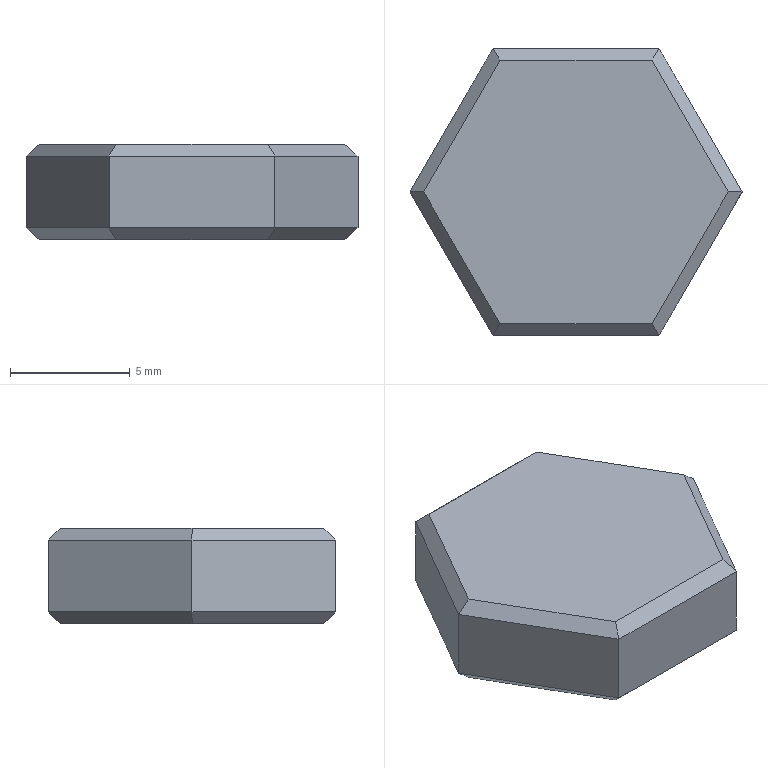Part | STEP file | Tube feed_id806_x_t | 1 solid | 20 faces | box 13.856 x 12 x 4 mm | volume 488.727 mm3 | plane 20
STEP:
#1=CARTESIAN_POINT('',(0.,0.,0.));
#2=DIRECTION('',(0.,0.,1.));
#3=DIRECTION('',(1.,0.,0.));
#4=AXIS2_PLACEMENT_3D('',#1,#2,#3);
#5=CARTESIAN_POINT('',(442.822,17.036,12.5));
#6=VERTEX_POINT('',#5);
#7=CARTESIAN_POINT('',(442.822,17.036,9.5));
#8=VERTEX_POINT('',#7);
#9=CARTESIAN_POINT('',(442.822,17.036,13.));
#10=DIRECTION('',(0.,0.,-1.));
#11=VECTOR('',#10,1.);
#12=LINE('',#9,#11);
#13=CARTESIAN_POINT('',(442.822,17.036,13.));
#14=DIRECTION('',(0.866,0.5,0.));
#15=DIRECTION('',(-0.5,0.866,0.));
#16=AXIS2_PLACEMENT_3D('',#13,#14,#15);
#17=PLANE('',#16);
#18=CARTESIAN_POINT('',(0.,0.));
#19=DIRECTION('',(0.,-1.));
#20=VECTOR('',#19,1.);
#21=LINE('',#18,#20);
#22=(GEOMETRIC_REPRESENTATION_CONTEXT(2)PARAMETRIC_REPRESENTATION_CONTEXT()REPRESENTATION_CONTEXT('',''));
#23=DEFINITIONAL_REPRESENTATION('',(#21),#22);
#24=PCURVE('',#17,#23);
#25=CARTESIAN_POINT('',(446.286,23.036,13.));
#26=DIRECTION('',(0.866,-0.5,0.));
#27=DIRECTION('',(0.5,0.866,0.));
#28=AXIS2_PLACEMENT_3D('',#25,#26,#27);
#29=PLANE('',#28);
#30=CARTESIAN_POINT('',(-6.928,0.));
#31=DIRECTION('',(0.,-1.));
#32=VECTOR('',#31,1.);
#33=LINE('',#30,#32);
#34=(GEOMETRIC_REPRESENTATION_CONTEXT(2)PARAMETRIC_REPRESENTATION_CONTEXT()REPRESENTATION_CONTEXT('',''));
#35=DEFINITIONAL_REPRESENTATION('',(#33),#34);
#36=PCURVE('',#29,#35);
#37=SURFACE_CURVE('',#12,(#24,#36),.PCURVE_S1.);
#38=EDGE_CURVE('',#6,#8,#37,.T.);
#39=ORIENTED_EDGE('',*,*,#38,.T.);
#40=CARTESIAN_POINT('',(446.286,11.036,9.5));
#41=VERTEX_POINT('',#40);
#42=CARTESIAN_POINT('',(442.822,17.036,9.5));
#43=DIRECTION('',(0.5,-0.866,0.));
#44=VECTOR('',#43,1.);
#45=LINE('',#42,#44);
#46=CARTESIAN_POINT('',(0.,-3.5));
#47=DIRECTION('',(-1.,0.));
#48=VECTOR('',#47,1.);
#49=LINE('',#46,#48);
#50=(GEOMETRIC_REPRESENTATION_CONTEXT(2)PARAMETRIC_REPRESENTATION_CONTEXT()REPRESENTATION_CONTEXT('',''));
#51=DEFINITIONAL_REPRESENTATION('',(#49),#50);
#52=PCURVE('',#17,#51);
#53=CARTESIAN_POINT('',(442.822,17.036,9.5));
#54=DIRECTION('',(0.6124,0.3536,0.7071));
#55=DIRECTION('',(0.5,-0.866,0.));
#56=AXIS2_PLACEMENT_3D('',#53,#54,#55);
#57=PLANE('',#56);
#58=CARTESIAN_POINT('',(0.,0.));
#59=DIRECTION('',(1.,0.));
#60=VECTOR('',#59,1.);
#61=LINE('',#58,#60);
#62=(GEOMETRIC_REPRESENTATION_CONTEXT(2)PARAMETRIC_REPRESENTATION_CONTEXT()REPRESENTATION_CONTEXT('',''));
#63=DEFINITIONAL_REPRESENTATION('',(#61),#62);
#64=PCURVE('',#57,#63);
#65=SURFACE_CURVE('',#45,(#52,#64),.PCURVE_S1.);
#66=EDGE_CURVE('',#8,#41,#65,.T.);
#67=ORIENTED_EDGE('',*,*,#66,.T.);
#68=CARTESIAN_POINT('',(446.286,11.036,12.5));
#69=VERTEX_POINT('',#68);
#70=CARTESIAN_POINT('',(446.286,11.036,13.));
#71=DIRECTION('',(0.,0.,-1.));
#72=VECTOR('',#71,1.);
#73=LINE('',#70,#72);
#74=CARTESIAN_POINT('',(-6.928,0.));
#75=DIRECTION('',(0.,-1.));
#76=VECTOR('',#75,1.);
#77=LINE('',#74,#76);
#78=(GEOMETRIC_REPRESENTATION_CONTEXT(2)PARAMETRIC_REPRESENTATION_CONTEXT()REPRESENTATION_CONTEXT('',''));
#79=DEFINITIONAL_REPRESENTATION('',(#77),#78);
#80=PCURVE('',#17,#79);
#81=CARTESIAN_POINT('',(446.286,11.036,13.));
#82=DIRECTION('',(0.,1.,0.));
#83=DIRECTION('',(-1.,0.,0.));
#84=AXIS2_PLACEMENT_3D('',#81,#82,#83);
#85=PLANE('',#84);
#86=CARTESIAN_POINT('',(0.,0.));
#87=DIRECTION('',(0.,-1.));
#88=VECTOR('',#87,1.);
#89=LINE('',#86,#88);
#90=(GEOMETRIC_REPRESENTATION_CONTEXT(2)PARAMETRIC_REPRESENTATION_CONTEXT()REPRESENTATION_CONTEXT('',''));
#91=DEFINITIONAL_REPRESENTATION('',(#89),#90);
#92=PCURVE('',#85,#91);
#93=SURFACE_CURVE('',#73,(#80,#92),.PCURVE_S1.);
#94=EDGE_CURVE('',#69,#41,#93,.T.);
#95=ORIENTED_EDGE('',*,*,#94,.F.);
#96=CARTESIAN_POINT('',(442.822,17.036,12.5));
#97=DIRECTION('',(-0.5,0.866,0.));
#98=VECTOR('',#97,1.);
#99=LINE('',#96,#98);
#100=CARTESIAN_POINT('',(0.,-0.5));
#101=DIRECTION('',(1.,0.));
#102=VECTOR('',#101,1.);
#103=LINE('',#100,#102);
#104=(GEOMETRIC_REPRESENTATION_CONTEXT(2)PARAMETRIC_REPRESENTATION_CONTEXT()REPRESENTATION_CONTEXT('',''));
#105=DEFINITIONAL_REPRESENTATION('',(#103),#104);
#106=PCURVE('',#17,#105);
#107=CARTESIAN_POINT('',(339.06,197.756,13.));
#108=DIRECTION('',(-0.6124,-0.3536,0.7071));
#109=DIRECTION('',(-0.5,0.866,0.));
#110=AXIS2_PLACEMENT_3D('',#107,#108,#109);
#111=PLANE('',#110);
#112=CARTESIAN_POINT('',(-208.39,0.7071));
#113=DIRECTION('',(1.,0.));
#114=VECTOR('',#113,1.);
#115=LINE('',#112,#114);
#116=(GEOMETRIC_REPRESENTATION_CONTEXT(2)PARAMETRIC_REPRESENTATION_CONTEXT()REPRESENTATION_CONTEXT('',''));
#117=DEFINITIONAL_REPRESENTATION('',(#115),#116);
#118=PCURVE('',#111,#117);
#119=SURFACE_CURVE('',#99,(#106,#118),.PCURVE_S1.);
#120=EDGE_CURVE('',#69,#6,#119,.T.);
#121=ORIENTED_EDGE('',*,*,#120,.T.);
#122=EDGE_LOOP('',(#39,#67,#95,#121));
#123=FACE_BOUND('',#122,.T.);
#124=ADVANCED_FACE('',(#123),#17,.F.);
#125=ORIENTED_EDGE('',*,*,#94,.T.);
#126=CARTESIAN_POINT('',(453.214,11.036,9.5));
#127=VERTEX_POINT('',#126);
#128=CARTESIAN_POINT('',(446.286,11.036,9.5));
#129=DIRECTION('',(1.,0.,0.));
#130=VECTOR('',#129,1.);
#131=LINE('',#128,#130);
#132=CARTESIAN_POINT('',(0.,-3.5));
#133=DIRECTION('',(-1.,0.));
#134=VECTOR('',#133,1.);
#135=LINE('',#132,#134);
#136=(GEOMETRIC_REPRESENTATION_CONTEXT(2)PARAMETRIC_REPRESENTATION_CONTEXT()REPRESENTATION_CONTEXT('',''));
#137=DEFINITIONAL_REPRESENTATION('',(#135),#136);
#138=PCURVE('',#85,#137);
#139=CARTESIAN_POINT('',(446.286,11.036,9.5));
#140=DIRECTION('',(0.,0.7071,0.7071));
#141=DIRECTION('',(1.,0.,0.));
#142=AXIS2_PLACEMENT_3D('',#139,#140,#141);
#143=PLANE('',#142);
#144=CARTESIAN_POINT('',(0.,0.));
#145=DIRECTION('',(1.,0.));
#146=VECTOR('',#145,1.);
#147=LINE('',#144,#146);
#148=(GEOMETRIC_REPRESENTATION_CONTEXT(2)PARAMETRIC_REPRESENTATION_CONTEXT()REPRESENTATION_CONTEXT('',''));
#149=DEFINITIONAL_REPRESENTATION('',(#147),#148);
#150=PCURVE('',#143,#149);
#151=SURFACE_CURVE('',#131,(#138,#150),.PCURVE_S1.);
#152=EDGE_CURVE('',#41,#127,#151,.T.);
#153=ORIENTED_EDGE('',*,*,#152,.T.);
#154=CARTESIAN_POINT('',(453.214,11.036,12.5));
#155=VERTEX_POINT('',#154);
#156=CARTESIAN_POINT('',(453.214,11.036,13.));
#157=DIRECTION('',(0.,0.,-1.));
#158=VECTOR('',#157,1.);
#159=LINE('',#156,#158);
#160=CARTESIAN_POINT('',(-6.928,0.));
#161=DIRECTION('',(0.,-1.));
#162=VECTOR('',#161,1.);
#163=LINE('',#160,#162);
#164=(GEOMETRIC_REPRESENTATION_CONTEXT(2)PARAMETRIC_REPRESENTATION_CONTEXT()REPRESENTATION_CONTEXT('',''));
#165=DEFINITIONAL_REPRESENTATION('',(#163),#164);
#166=PCURVE('',#85,#165);
#167=CARTESIAN_POINT('',(453.214,11.036,13.));
#168=DIRECTION('',(-0.866,0.5,0.));
#169=DIRECTION('',(-0.5,-0.866,0.));
#170=AXIS2_PLACEMENT_3D('',#167,#168,#169);
#171=PLANE('',#170);
#172=CARTESIAN_POINT('',(0.,0.));
#173=DIRECTION('',(0.,-1.));
#174=VECTOR('',#173,1.);
#175=LINE('',#172,#174);
#176=(GEOMETRIC_REPRESENTATION_CONTEXT(2)PARAMETRIC_REPRESENTATION_CONTEXT()REPRESENTATION_CONTEXT('',''));
#177=DEFINITIONAL_REPRESENTATION('',(#175),#176);
#178=PCURVE('',#171,#177);
#179=SURFACE_CURVE('',#159,(#166,#178),.PCURVE_S1.);
#180=EDGE_CURVE('',#155,#127,#179,.T.);
#181=ORIENTED_EDGE('',*,*,#180,.F.);
#182=CARTESIAN_POINT('',(446.286,11.036,12.5));
#183=DIRECTION('',(-1.,0.,0.));
#184=VECTOR('',#183,1.);
#185=LINE('',#182,#184);
#186=CARTESIAN_POINT('',(0.,-0.5));
#187=DIRECTION('',(1.,0.));
#188=VECTOR('',#187,1.);
#189=LINE('',#186,#188);
#190=(GEOMETRIC_REPRESENTATION_CONTEXT(2)PARAMETRIC_REPRESENTATION_CONTEXT()REPRESENTATION_CONTEXT('',''));
#191=DEFINITIONAL_REPRESENTATION('',(#189),#190);
#192=PCURVE('',#85,#191);
#193=CARTESIAN_POINT('',(0.,11.536,13.));
#194=DIRECTION('',(0.,-0.7071,0.7071));
#195=DIRECTION('',(-1.,0.,0.));
#196=AXIS2_PLACEMENT_3D('',#193,#194,#195);
#197=PLANE('',#196);
#198=CARTESIAN_POINT('',(-446.286,0.7071));
#199=DIRECTION('',(1.,0.));
#200=VECTOR('',#199,1.);
#201=LINE('',#198,#200);
#202=(GEOMETRIC_REPRESENTATION_CONTEXT(2)PARAMETRIC_REPRESENTATION_CONTEXT()REPRESENTATION_CONTEXT('',''));
#203=DEFINITIONAL_REPRESENTATION('',(#201),#202);
#204=PCURVE('',#197,#203);
#205=SURFACE_CURVE('',#185,(#192,#204),.PCURVE_S1.);
#206=EDGE_CURVE('',#155,#69,#205,.T.);
#207=ORIENTED_EDGE('',*,*,#206,.T.);
#208=EDGE_LOOP('',(#125,#153,#181,#207));
#209=FACE_BOUND('',#208,.T.);
#210=ADVANCED_FACE('',(#209),#85,.F.);
#211=ORIENTED_EDGE('',*,*,#180,.T.);
#212=CARTESIAN_POINT('',(456.678,17.036,9.5));
#213=VERTEX_POINT('',#212);
#214=CARTESIAN_POINT('',(453.214,11.036,9.5));
#215=DIRECTION('',(0.5,0.866,0.));
#216=VECTOR('',#215,1.);
#217=LINE('',#214,#216);
#218=CARTESIAN_POINT('',(0.,-3.5));
#219=DIRECTION('',(-1.,0.));
#220=VECTOR('',#219,1.);
#221=LINE('',#218,#220);
#222=(GEOMETRIC_REPRESENTATION_CONTEXT(2)PARAMETRIC_REPRESENTATION_CONTEXT()REPRESENTATION_CONTEXT('',''));
#223=DEFINITIONAL_REPRESENTATION('',(#221),#222);
#224=PCURVE('',#171,#223);
#225=CARTESIAN_POINT('',(453.214,11.036,9.5));
#226=DIRECTION('',(-0.6124,0.3536,0.7071));
#227=DIRECTION('',(0.5,0.866,0.));
#228=AXIS2_PLACEMENT_3D('',#225,#226,#227);
#229=PLANE('',#228);
#230=CARTESIAN_POINT('',(0.,0.));
#231=DIRECTION('',(1.,0.));
#232=VECTOR('',#231,1.);
#233=LINE('',#230,#232);
#234=(GEOMETRIC_REPRESENTATION_CONTEXT(2)PARAMETRIC_REPRESENTATION_CONTEXT()REPRESENTATION_CONTEXT('',''));
#235=DEFINITIONAL_REPRESENTATION('',(#233),#234);
#236=PCURVE('',#229,#235);
#237=SURFACE_CURVE('',#217,(#224,#236),.PCURVE_S1.);
#238=EDGE_CURVE('',#127,#213,#237,.T.);
#239=ORIENTED_EDGE('',*,*,#238,.T.);
#240=CARTESIAN_POINT('',(456.678,17.036,12.5));
#241=VERTEX_POINT('',#240);
#242=CARTESIAN_POINT('',(456.678,17.036,13.));
#243=DIRECTION('',(0.,0.,-1.));
#244=VECTOR('',#243,1.);
#245=LINE('',#242,#244);
#246=CARTESIAN_POINT('',(-6.928,0.));
#247=DIRECTION('',(0.,-1.));
#248=VECTOR('',#247,1.);
#249=LINE('',#246,#248);
#250=(GEOMETRIC_REPRESENTATION_CONTEXT(2)PARAMETRIC_REPRESENTATION_CONTEXT()REPRESENTATION_CONTEXT('',''));
#251=DEFINITIONAL_REPRESENTATION('',(#249),#250);
#252=PCURVE('',#171,#251);
#253=CARTESIAN_POINT('',(456.678,17.036,13.));
#254=DIRECTION('',(-0.866,-0.5,0.));
#255=DIRECTION('',(0.5,-0.866,0.));
#256=AXIS2_PLACEMENT_3D('',#253,#254,#255);
#257=PLANE('',#256);
#258=CARTESIAN_POINT('',(0.,0.));
#259=DIRECTION('',(0.,-1.));
#260=VECTOR('',#259,1.);
#261=LINE('',#258,#260);
#262=(GEOMETRIC_REPRESENTATION_CONTEXT(2)PARAMETRIC_REPRESENTATION_CONTEXT()REPRESENTATION_CONTEXT('',''));
#263=DEFINITIONAL_REPRESENTATION('',(#261),#262);
#264=PCURVE('',#257,#263);
#265=SURFACE_CURVE('',#245,(#252,#264),.PCURVE_S1.);
#266=EDGE_CURVE('',#241,#213,#265,.T.);
#267=ORIENTED_EDGE('',*,*,#266,.F.);
#268=CARTESIAN_POINT('',(453.214,11.036,12.5));
#269=DIRECTION('',(-0.5,-0.866,0.));
#270=VECTOR('',#269,1.);
#271=LINE('',#268,#270);
#272=CARTESIAN_POINT('',(0.,-0.5));
#273=DIRECTION('',(1.,0.));
#274=VECTOR('',#273,1.);
#275=LINE('',#272,#274);
#276=(GEOMETRIC_REPRESENTATION_CONTEXT(2)PARAMETRIC_REPRESENTATION_CONTEXT()REPRESENTATION_CONTEXT('',''));
#277=DEFINITIONAL_REPRESENTATION('',(#275),#276);
#278=PCURVE('',#171,#277);
#279=CARTESIAN_POINT('',(335.565,-191.739,13.));
#280=DIRECTION('',(0.6124,-0.3536,0.7071));
#281=DIRECTION('',(-0.5,-0.866,0.));
#282=AXIS2_PLACEMENT_3D('',#279,#280,#281);
#283=PLANE('',#282);
#284=CARTESIAN_POINT('',(-234.432,0.7071));
#285=DIRECTION('',(1.,0.));
#286=VECTOR('',#285,1.);
#287=LINE('',#284,#286);
#288=(GEOMETRIC_REPRESENTATION_CONTEXT(2)PARAMETRIC_REPRESENTATION_CONTEXT()REPRESENTATION_CONTEXT('',''));
#289=DEFINITIONAL_REPRESENTATION('',(#287),#288);
#290=PCURVE('',#283,#289);
#291=SURFACE_CURVE('',#271,(#278,#290),.PCURVE_S1.);
#292=EDGE_CURVE('',#241,#155,#291,.T.);
#293=ORIENTED_EDGE('',*,*,#292,.T.);
#294=EDGE_LOOP('',(#211,#239,#267,#293));
#295=FACE_BOUND('',#294,.T.);
#296=ADVANCED_FACE('',(#295),#171,.F.);
#297=ORIENTED_EDGE('',*,*,#266,.T.);
#298=CARTESIAN_POINT('',(453.214,23.036,9.5));
#299=VERTEX_POINT('',#298);
#300=CARTESIAN_POINT('',(456.678,17.036,9.5));
#301=DIRECTION('',(-0.5,0.866,0.));
#302=VECTOR('',#301,1.);
#303=LINE('',#300,#302);
#304=CARTESIAN_POINT('',(0.,-3.5));
#305=DIRECTION('',(-1.,0.));
#306=VECTOR('',#305,1.);
#307=LINE('',#304,#306);
#308=(GEOMETRIC_REPRESENTATION_CONTEXT(2)PARAMETRIC_REPRESENTATION_CONTEXT()REPRESENTATION_CONTEXT('',''));
#309=DEFINITIONAL_REPRESENTATION('',(#307),#308);
#310=PCURVE('',#257,#309);
#311=CARTESIAN_POINT('',(456.678,17.036,9.5));
#312=DIRECTION('',(-0.6124,-0.3536,0.7071));
#313=DIRECTION('',(-0.5,0.866,0.));
#314=AXIS2_PLACEMENT_3D('',#311,#312,#313);
#315=PLANE('',#314);
#316=CARTESIAN_POINT('',(0.,0.));
#317=DIRECTION('',(1.,0.));
#318=VECTOR('',#317,1.);
#319=LINE('',#316,#318);
#320=(GEOMETRIC_REPRESENTATION_CONTEXT(2)PARAMETRIC_REPRESENTATION_CONTEXT()REPRESENTATION_CONTEXT('',''));
#321=DEFINITIONAL_REPRESENTATION('',(#319),#320);
#322=PCURVE('',#315,#321);
#323=SURFACE_CURVE('',#303,(#310,#322),.PCURVE_S1.);
#324=EDGE_CURVE('',#213,#299,#323,.T.);
#325=ORIENTED_EDGE('',*,*,#324,.T.);
#326=CARTESIAN_POINT('',(453.214,23.036,12.5));
#327=VERTEX_POINT('',#326);
#328=CARTESIAN_POINT('',(453.214,23.036,13.));
#329=DIRECTION('',(0.,0.,-1.));
#330=VECTOR('',#329,1.);
#331=LINE('',#328,#330);
#332=CARTESIAN_POINT('',(-6.928,0.));
#333=DIRECTION('',(0.,-1.));
#334=VECTOR('',#333,1.);
#335=LINE('',#332,#334);
#336=(GEOMETRIC_REPRESENTATION_CONTEXT(2)PARAMETRIC_REPRESENTATION_CONTEXT()REPRESENTATION_CONTEXT('',''));
#337=DEFINITIONAL_REPRESENTATION('',(#335),#336);
#338=PCURVE('',#257,#337);
#339=CARTESIAN_POINT('',(453.214,23.036,13.));
#340=DIRECTION('',(0.,-1.,0.));
#341=DIRECTION('',(1.,0.,0.));
#342=AXIS2_PLACEMENT_3D('',#339,#340,#341);
#343=PLANE('',#342);
#344=CARTESIAN_POINT('',(0.,0.));
#345=DIRECTION('',(0.,-1.));
#346=VECTOR('',#345,1.);
#347=LINE('',#344,#346);
#348=(GEOMETRIC_REPRESENTATION_CONTEXT(2)PARAMETRIC_REPRESENTATION_CONTEXT()REPRESENTATION_CONTEXT('',''));
#349=DEFINITIONAL_REPRESENTATION('',(#347),#348);
#350=PCURVE('',#343,#349);
#351=SURFACE_CURVE('',#331,(#338,#350),.PCURVE_S1.);
#352=EDGE_CURVE('',#327,#299,#351,.T.);
#353=ORIENTED_EDGE('',*,*,#352,.F.);
#354=CARTESIAN_POINT('',(456.678,17.036,12.5));
#355=DIRECTION('',(0.5,-0.866,0.));
#356=VECTOR('',#355,1.);
#357=LINE('',#354,#356);
#358=CARTESIAN_POINT('',(0.,-0.5));
#359=DIRECTION('',(1.,0.));
#360=VECTOR('',#359,1.);
#361=LINE('',#358,#360);
#362=(GEOMETRIC_REPRESENTATION_CONTEXT(2)PARAMETRIC_REPRESENTATION_CONTEXT()REPRESENTATION_CONTEXT('',''));
#363=DEFINITIONAL_REPRESENTATION('',(#361),#362);
#364=PCURVE('',#257,#363);
#365=CARTESIAN_POINT('',(348.586,203.256,13.));
#366=DIRECTION('',(0.6124,0.3536,0.7071));
#367=DIRECTION('',(0.5,-0.866,0.));
#368=AXIS2_PLACEMENT_3D('',#365,#366,#367);
#369=PLANE('',#368);
#370=CARTESIAN_POINT('',(215.318,0.7071));
#371=DIRECTION('',(1.,0.));
#372=VECTOR('',#371,1.);
#373=LINE('',#370,#372);
#374=(GEOMETRIC_REPRESENTATION_CONTEXT(2)PARAMETRIC_REPRESENTATION_CONTEXT()REPRESENTATION_CONTEXT('',''));
#375=DEFINITIONAL_REPRESENTATION('',(#373),#374);
#376=PCURVE('',#369,#375);
#377=SURFACE_CURVE('',#357,(#364,#376),.PCURVE_S1.);
#378=EDGE_CURVE('',#327,#241,#377,.T.);
#379=ORIENTED_EDGE('',*,*,#378,.T.);
#380=EDGE_LOOP('',(#297,#325,#353,#379));
#381=FACE_BOUND('',#380,.T.);
#382=ADVANCED_FACE('',(#381),#257,.F.);
#383=ORIENTED_EDGE('',*,*,#352,.T.);
#384=CARTESIAN_POINT('',(446.286,23.036,9.5));
#385=VERTEX_POINT('',#384);
#386=CARTESIAN_POINT('',(453.214,23.036,9.5));
#387=DIRECTION('',(-1.,0.,0.));
#388=VECTOR('',#387,1.);
#389=LINE('',#386,#388);
#390=CARTESIAN_POINT('',(0.,-3.5));
#391=DIRECTION('',(-1.,0.));
#392=VECTOR('',#391,1.);
#393=LINE('',#390,#392);
#394=(GEOMETRIC_REPRESENTATION_CONTEXT(2)PARAMETRIC_REPRESENTATION_CONTEXT()REPRESENTATION_CONTEXT('',''));
#395=DEFINITIONAL_REPRESENTATION('',(#393),#394);
#396=PCURVE('',#343,#395);
#397=CARTESIAN_POINT('',(453.214,23.036,9.5));
#398=DIRECTION('',(0.,-0.7071,0.7071));
#399=DIRECTION('',(-1.,0.,0.));
#400=AXIS2_PLACEMENT_3D('',#397,#398,#399);
#401=PLANE('',#400);
#402=CARTESIAN_POINT('',(0.,0.));
#403=DIRECTION('',(1.,0.));
#404=VECTOR('',#403,1.);
#405=LINE('',#402,#404);
#406=(GEOMETRIC_REPRESENTATION_CONTEXT(2)PARAMETRIC_REPRESENTATION_CONTEXT()REPRESENTATION_CONTEXT('',''));
#407=DEFINITIONAL_REPRESENTATION('',(#405),#406);
#408=PCURVE('',#401,#407);
#409=SURFACE_CURVE('',#389,(#396,#408),.PCURVE_S1.);
#410=EDGE_CURVE('',#299,#385,#409,.T.);
#411=ORIENTED_EDGE('',*,*,#410,.T.);
#412=CARTESIAN_POINT('',(446.286,23.036,12.5));
#413=VERTEX_POINT('',#412);
#414=CARTESIAN_POINT('',(446.286,23.036,13.));
#415=DIRECTION('',(0.,0.,-1.));
#416=VECTOR('',#415,1.);
#417=LINE('',#414,#416);
#418=CARTESIAN_POINT('',(-6.928,0.));
#419=DIRECTION('',(0.,-1.));
#420=VECTOR('',#419,1.);
#421=LINE('',#418,#420);
#422=(GEOMETRIC_REPRESENTATION_CONTEXT(2)PARAMETRIC_REPRESENTATION_CONTEXT()REPRESENTATION_CONTEXT('',''));
#423=DEFINITIONAL_REPRESENTATION('',(#421),#422);
#424=PCURVE('',#343,#423);
#425=CARTESIAN_POINT('',(0.,0.));
#426=DIRECTION('',(0.,-1.));
#427=VECTOR('',#426,1.);
#428=LINE('',#425,#427);
#429=(GEOMETRIC_REPRESENTATION_CONTEXT(2)PARAMETRIC_REPRESENTATION_CONTEXT()REPRESENTATION_CONTEXT('',''));
#430=DEFINITIONAL_REPRESENTATION('',(#428),#429);
#431=PCURVE('',#29,#430);
#432=SURFACE_CURVE('',#417,(#424,#431),.PCURVE_S1.);
#433=EDGE_CURVE('',#413,#385,#432,.T.);
#434=ORIENTED_EDGE('',*,*,#433,.F.);
#435=CARTESIAN_POINT('',(453.214,23.036,12.5));
#436=DIRECTION('',(1.,0.,0.));
#437=VECTOR('',#436,1.);
#438=LINE('',#435,#437);
#439=CARTESIAN_POINT('',(0.,-0.5));
#440=DIRECTION('',(1.,0.));
#441=VECTOR('',#440,1.);
#442=LINE('',#439,#441);
#443=(GEOMETRIC_REPRESENTATION_CONTEXT(2)PARAMETRIC_REPRESENTATION_CONTEXT()REPRESENTATION_CONTEXT('',''));
#444=DEFINITIONAL_REPRESENTATION('',(#442),#443);
#445=PCURVE('',#343,#444);
#446=CARTESIAN_POINT('',(0.,22.536,13.));
#447=DIRECTION('',(0.,0.7071,0.7071));
#448=DIRECTION('',(1.,0.,0.));
#449=AXIS2_PLACEMENT_3D('',#446,#447,#448);
#450=PLANE('',#449);
#451=CARTESIAN_POINT('',(453.214,0.7071));
#452=DIRECTION('',(1.,0.));
#453=VECTOR('',#452,1.);
#454=LINE('',#451,#453);
#455=(GEOMETRIC_REPRESENTATION_CONTEXT(2)PARAMETRIC_REPRESENTATION_CONTEXT()REPRESENTATION_CONTEXT('',''));
#456=DEFINITIONAL_REPRESENTATION('',(#454),#455);
#457=PCURVE('',#450,#456);
#458=SURFACE_CURVE('',#438,(#445,#457),.PCURVE_S1.);
#459=EDGE_CURVE('',#413,#327,#458,.T.);
#460=ORIENTED_EDGE('',*,*,#459,.T.);
#461=EDGE_LOOP('',(#383,#411,#434,#460));
#462=FACE_BOUND('',#461,.T.);
#463=ADVANCED_FACE('',(#462),#343,.F.);
#464=ORIENTED_EDGE('',*,*,#433,.T.);
#465=CARTESIAN_POINT('',(446.286,23.036,9.5));
#466=DIRECTION('',(-0.5,-0.866,0.));
#467=VECTOR('',#466,1.);
#468=LINE('',#465,#467);
#469=CARTESIAN_POINT('',(0.,-3.5));
#470=DIRECTION('',(-1.,0.));
#471=VECTOR('',#470,1.);
#472=LINE('',#469,#471);
#473=(GEOMETRIC_REPRESENTATION_CONTEXT(2)PARAMETRIC_REPRESENTATION_CONTEXT()REPRESENTATION_CONTEXT('',''));
#474=DEFINITIONAL_REPRESENTATION('',(#472),#473);
#475=PCURVE('',#29,#474);
#476=CARTESIAN_POINT('',(446.286,23.036,9.5));
#477=DIRECTION('',(0.6124,-0.3536,0.7071));
#478=DIRECTION('',(-0.5,-0.866,0.));
#479=AXIS2_PLACEMENT_3D('',#476,#477,#478);
#480=PLANE('',#479);
#481=CARTESIAN_POINT('',(0.,0.));
#482=DIRECTION('',(1.,0.));
#483=VECTOR('',#482,1.);
#484=LINE('',#481,#483);
#485=(GEOMETRIC_REPRESENTATION_CONTEXT(2)PARAMETRIC_REPRESENTATION_CONTEXT()REPRESENTATION_CONTEXT('',''));
#486=DEFINITIONAL_REPRESENTATION('',(#484),#485);
#487=PCURVE('',#480,#486);
#488=SURFACE_CURVE('',#468,(#475,#487),.PCURVE_S1.);
#489=EDGE_CURVE('',#385,#8,#488,.T.);
#490=ORIENTED_EDGE('',*,*,#489,.T.);
#491=ORIENTED_EDGE('',*,*,#38,.F.);
#492=CARTESIAN_POINT('',(446.286,23.036,12.5));
#493=DIRECTION('',(0.5,0.866,0.));
#494=VECTOR('',#493,1.);
#495=LINE('',#492,#494);
#496=CARTESIAN_POINT('',(0.,-0.5));
#497=DIRECTION('',(1.,0.));
#498=VECTOR('',#497,1.);
#499=LINE('',#496,#498);
#500=(GEOMETRIC_REPRESENTATION_CONTEXT(2)PARAMETRIC_REPRESENTATION_CONTEXT()REPRESENTATION_CONTEXT('',''));
#501=DEFINITIONAL_REPRESENTATION('',(#499),#500);
#502=PCURVE('',#29,#501);
#503=CARTESIAN_POINT('',(326.039,-186.239,13.));
#504=DIRECTION('',(-0.6124,0.3536,0.7071));
#505=DIRECTION('',(0.5,0.866,0.));
#506=AXIS2_PLACEMENT_3D('',#503,#504,#505);
#507=PLANE('',#506);
#508=CARTESIAN_POINT('',(241.36,0.7071));
#509=DIRECTION('',(1.,0.));
#510=VECTOR('',#509,1.);
#511=LINE('',#508,#510);
#512=(GEOMETRIC_REPRESENTATION_CONTEXT(2)PARAMETRIC_REPRESENTATION_CONTEXT()REPRESENTATION_CONTEXT('',''));
#513=DEFINITIONAL_REPRESENTATION('',(#511),#512);
#514=PCURVE('',#507,#513);
#515=SURFACE_CURVE('',#495,(#502,#514),.PCURVE_S1.);
#516=EDGE_CURVE('',#6,#413,#515,.T.);
#517=ORIENTED_EDGE('',*,*,#516,.T.);
#518=EDGE_LOOP('',(#464,#490,#491,#517));
#519=FACE_BOUND('',#518,.T.);
#520=ADVANCED_FACE('',(#519),#29,.F.);
#521=CARTESIAN_POINT('',(446.575,22.536,13.));
#522=VERTEX_POINT('',#521);
#523=CARTESIAN_POINT('',(443.399,17.036,13.));
#524=VERTEX_POINT('',#523);
#525=CARTESIAN_POINT('',(443.255,16.786,13.));
#526=DIRECTION('',(-0.5,-0.866,0.));
#527=VECTOR('',#526,1.);
#528=LINE('',#525,#527);
#529=CARTESIAN_POINT('',(0.,2.,13.));
#530=DIRECTION('',(0.,0.,1.));
#531=DIRECTION('',(1.,0.,0.));
#532=AXIS2_PLACEMENT_3D('',#529,#530,#531);
#533=PLANE('',#532);
#534=CARTESIAN_POINT('',(443.255,14.786));
#535=DIRECTION('',(-0.5,-0.866));
#536=VECTOR('',#535,1.);
#537=LINE('',#534,#536);
#538=(GEOMETRIC_REPRESENTATION_CONTEXT(2)PARAMETRIC_REPRESENTATION_CONTEXT()REPRESENTATION_CONTEXT('',''));
#539=DEFINITIONAL_REPRESENTATION('',(#537),#538);
#540=PCURVE('',#533,#539);
#541=CARTESIAN_POINT('',(234.432,0.));
#542=DIRECTION('',(-1.,0.));
#543=VECTOR('',#542,1.);
#544=LINE('',#541,#543);
#545=(GEOMETRIC_REPRESENTATION_CONTEXT(2)PARAMETRIC_REPRESENTATION_CONTEXT()REPRESENTATION_CONTEXT('',''));
#546=DEFINITIONAL_REPRESENTATION('',(#544),#545);
#547=PCURVE('',#507,#546);
#548=SURFACE_CURVE('',#528,(#540,#547),.PCURVE_S1.);
#549=EDGE_CURVE('',#522,#524,#548,.T.);
#550=ORIENTED_EDGE('',*,*,#549,.T.);
#551=CARTESIAN_POINT('',(446.575,11.536,13.));
#552=VERTEX_POINT('',#551);
#553=CARTESIAN_POINT('',(446.719,11.286,13.));
#554=DIRECTION('',(0.5,-0.866,0.));
#555=VECTOR('',#554,1.);
#556=LINE('',#553,#555);
#557=CARTESIAN_POINT('',(446.719,9.286));
#558=DIRECTION('',(0.5,-0.866));
#559=VECTOR('',#558,1.);
#560=LINE('',#557,#559);
#561=(GEOMETRIC_REPRESENTATION_CONTEXT(2)PARAMETRIC_REPRESENTATION_CONTEXT()REPRESENTATION_CONTEXT('',''));
#562=DEFINITIONAL_REPRESENTATION('',(#560),#561);
#563=PCURVE('',#533,#562);
#564=CARTESIAN_POINT('',(-215.318,0.));
#565=DIRECTION('',(-1.,0.));
#566=VECTOR('',#565,1.);
#567=LINE('',#564,#566);
#568=(GEOMETRIC_REPRESENTATION_CONTEXT(2)PARAMETRIC_REPRESENTATION_CONTEXT()REPRESENTATION_CONTEXT('',''));
#569=DEFINITIONAL_REPRESENTATION('',(#567),#568);
#570=PCURVE('',#111,#569);
#571=SURFACE_CURVE('',#556,(#563,#570),.PCURVE_S1.);
#572=EDGE_CURVE('',#524,#552,#571,.T.);
#573=ORIENTED_EDGE('',*,*,#572,.T.);
#574=CARTESIAN_POINT('',(452.925,11.536,13.));
#575=VERTEX_POINT('',#574);
#576=CARTESIAN_POINT('',(453.214,11.536,13.));
#577=DIRECTION('',(1.,0.,0.));
#578=VECTOR('',#577,1.);
#579=LINE('',#576,#578);
#580=CARTESIAN_POINT('',(453.214,9.536));
#581=DIRECTION('',(1.,0.));
#582=VECTOR('',#581,1.);
#583=LINE('',#580,#582);
#584=(GEOMETRIC_REPRESENTATION_CONTEXT(2)PARAMETRIC_REPRESENTATION_CONTEXT()REPRESENTATION_CONTEXT('',''));
#585=DEFINITIONAL_REPRESENTATION('',(#583),#584);
#586=PCURVE('',#533,#585);
#587=CARTESIAN_POINT('',(-453.214,0.));
#588=DIRECTION('',(-1.,0.));
#589=VECTOR('',#588,1.);
#590=LINE('',#587,#589);
#591=(GEOMETRIC_REPRESENTATION_CONTEXT(2)PARAMETRIC_REPRESENTATION_CONTEXT()REPRESENTATION_CONTEXT('',''));
#592=DEFINITIONAL_REPRESENTATION('',(#590),#591);
#593=PCURVE('',#197,#592);
#594=SURFACE_CURVE('',#579,(#586,#593),.PCURVE_S1.);
#595=EDGE_CURVE('',#552,#575,#594,.T.);
#596=ORIENTED_EDGE('',*,*,#595,.T.);
#597=CARTESIAN_POINT('',(456.101,17.036,13.));
#598=VERTEX_POINT('',#597);
#599=CARTESIAN_POINT('',(456.245,17.286,13.));
#600=DIRECTION('',(0.5,0.866,0.));
#601=VECTOR('',#600,1.);
#602=LINE('',#599,#601);
#603=CARTESIAN_POINT('',(456.245,15.286));
#604=DIRECTION('',(0.5,0.866));
#605=VECTOR('',#604,1.);
#606=LINE('',#603,#605);
#607=(GEOMETRIC_REPRESENTATION_CONTEXT(2)PARAMETRIC_REPRESENTATION_CONTEXT()REPRESENTATION_CONTEXT('',''));
#608=DEFINITIONAL_REPRESENTATION('',(#606),#607);
#609=PCURVE('',#533,#608);
#610=CARTESIAN_POINT('',(-241.36,0.));
#611=DIRECTION('',(-1.,0.));
#612=VECTOR('',#611,1.);
#613=LINE('',#610,#612);
#614=(GEOMETRIC_REPRESENTATION_CONTEXT(2)PARAMETRIC_REPRESENTATION_CONTEXT()REPRESENTATION_CONTEXT('',''));
#615=DEFINITIONAL_REPRESENTATION('',(#613),#614);
#616=PCURVE('',#283,#615);
#617=SURFACE_CURVE('',#602,(#609,#616),.PCURVE_S1.);
#618=EDGE_CURVE('',#575,#598,#617,.T.);
#619=ORIENTED_EDGE('',*,*,#618,.T.);
#620=CARTESIAN_POINT('',(452.925,22.536,13.));
#621=VERTEX_POINT('',#620);
#622=CARTESIAN_POINT('',(452.781,22.786,13.));
#623=DIRECTION('',(-0.5,0.866,0.));
#624=VECTOR('',#623,1.);
#625=LINE('',#622,#624);
#626=CARTESIAN_POINT('',(452.781,20.786));
#627=DIRECTION('',(-0.5,0.866));
#628=VECTOR('',#627,1.);
#629=LINE('',#626,#628);
#630=(GEOMETRIC_REPRESENTATION_CONTEXT(2)PARAMETRIC_REPRESENTATION_CONTEXT()REPRESENTATION_CONTEXT('',''));
#631=DEFINITIONAL_REPRESENTATION('',(#629),#630);
#632=PCURVE('',#533,#631);
#633=CARTESIAN_POINT('',(208.39,0.));
#634=DIRECTION('',(-1.,0.));
#635=VECTOR('',#634,1.);
#636=LINE('',#633,#635);
#637=(GEOMETRIC_REPRESENTATION_CONTEXT(2)PARAMETRIC_REPRESENTATION_CONTEXT()REPRESENTATION_CONTEXT('',''));
#638=DEFINITIONAL_REPRESENTATION('',(#636),#637);
#639=PCURVE('',#369,#638);
#640=SURFACE_CURVE('',#625,(#632,#639),.PCURVE_S1.);
#641=EDGE_CURVE('',#598,#621,#640,.T.);
#642=ORIENTED_EDGE('',*,*,#641,.T.);
#643=CARTESIAN_POINT('',(446.286,22.536,13.));
#644=DIRECTION('',(-1.,0.,0.));
#645=VECTOR('',#644,1.);
#646=LINE('',#643,#645);
#647=CARTESIAN_POINT('',(446.286,20.536));
#648=DIRECTION('',(-1.,0.));
#649=VECTOR('',#648,1.);
#650=LINE('',#647,#649);
#651=(GEOMETRIC_REPRESENTATION_CONTEXT(2)PARAMETRIC_REPRESENTATION_CONTEXT()REPRESENTATION_CONTEXT('',''));
#652=DEFINITIONAL_REPRESENTATION('',(#650),#651);
#653=PCURVE('',#533,#652);
#654=CARTESIAN_POINT('',(446.286,0.));
#655=DIRECTION('',(-1.,0.));
#656=VECTOR('',#655,1.);
#657=LINE('',#654,#656);
#658=(GEOMETRIC_REPRESENTATION_CONTEXT(2)PARAMETRIC_REPRESENTATION_CONTEXT()REPRESENTATION_CONTEXT('',''));
#659=DEFINITIONAL_REPRESENTATION('',(#657),#658);
#660=PCURVE('',#450,#659);
#661=SURFACE_CURVE('',#646,(#653,#660),.PCURVE_S1.);
#662=EDGE_CURVE('',#621,#522,#661,.T.);
#663=ORIENTED_EDGE('',*,*,#662,.T.);
#664=EDGE_LOOP('',(#550,#573,#596,#619,#642,#663));
#665=FACE_BOUND('',#664,.T.);
#666=ADVANCED_FACE('',(#665),#533,.T.);
#667=CARTESIAN_POINT('',(452.925,11.536,9.));
#668=VERTEX_POINT('',#667);
#669=CARTESIAN_POINT('',(446.575,11.536,9.));
#670=VERTEX_POINT('',#669);
#671=CARTESIAN_POINT('',(0.,11.536,9.));
#672=DIRECTION('',(-1.,0.,0.));
#673=VECTOR('',#672,1.);
#674=LINE('',#671,#673);
#675=CARTESIAN_POINT('',(0.,2.,9.));
#676=DIRECTION('',(0.,0.,1.));
#677=DIRECTION('',(1.,0.,0.));
#678=AXIS2_PLACEMENT_3D('',#675,#676,#677);
#679=PLANE('',#678);
#680=CARTESIAN_POINT('',(0.,9.536));
#681=DIRECTION('',(-1.,0.));
#682=VECTOR('',#681,1.);
#683=LINE('',#680,#682);
#684=(GEOMETRIC_REPRESENTATION_CONTEXT(2)PARAMETRIC_REPRESENTATION_CONTEXT()REPRESENTATION_CONTEXT('',''));
#685=DEFINITIONAL_REPRESENTATION('',(#683),#684);
#686=PCURVE('',#679,#685);
#687=CARTESIAN_POINT('',(-446.286,0.7071));
#688=DIRECTION('',(-1.,0.));
#689=VECTOR('',#688,1.);
#690=LINE('',#687,#689);
#691=(GEOMETRIC_REPRESENTATION_CONTEXT(2)PARAMETRIC_REPRESENTATION_CONTEXT()REPRESENTATION_CONTEXT('',''));
#692=DEFINITIONAL_REPRESENTATION('',(#690),#691);
#693=PCURVE('',#143,#692);
#694=SURFACE_CURVE('',#674,(#686,#693),.PCURVE_S1.);
#695=EDGE_CURVE('',#668,#670,#694,.T.);
#696=ORIENTED_EDGE('',*,*,#695,.T.);
#697=CARTESIAN_POINT('',(443.399,17.036,9.));
#698=VERTEX_POINT('',#697);
#699=CARTESIAN_POINT('',(339.06,197.756,9.));
#700=DIRECTION('',(-0.5,0.866,0.));
#701=VECTOR('',#700,1.);
#702=LINE('',#699,#701);
#703=CARTESIAN_POINT('',(339.06,195.756));
#704=DIRECTION('',(-0.5,0.866));
#705=VECTOR('',#704,1.);
#706=LINE('',#703,#705);
#707=(GEOMETRIC_REPRESENTATION_CONTEXT(2)PARAMETRIC_REPRESENTATION_CONTEXT()REPRESENTATION_CONTEXT('',''));
#708=DEFINITIONAL_REPRESENTATION('',(#706),#707);
#709=PCURVE('',#679,#708);
#710=CARTESIAN_POINT('',(-208.39,0.7071));
#711=DIRECTION('',(-1.,0.));
#712=VECTOR('',#711,1.);
#713=LINE('',#710,#712);
#714=(GEOMETRIC_REPRESENTATION_CONTEXT(2)PARAMETRIC_REPRESENTATION_CONTEXT()REPRESENTATION_CONTEXT('',''));
#715=DEFINITIONAL_REPRESENTATION('',(#713),#714);
#716=PCURVE('',#57,#715);
#717=SURFACE_CURVE('',#702,(#709,#716),.PCURVE_S1.);
#718=EDGE_CURVE('',#670,#698,#717,.T.);
#719=ORIENTED_EDGE('',*,*,#718,.T.);
#720=CARTESIAN_POINT('',(446.575,22.536,9.));
#721=VERTEX_POINT('',#720);
#722=CARTESIAN_POINT('',(326.039,-186.239,9.));
#723=DIRECTION('',(0.5,0.866,0.));
#724=VECTOR('',#723,1.);
#725=LINE('',#722,#724);
#726=CARTESIAN_POINT('',(326.039,-188.239));
#727=DIRECTION('',(0.5,0.866));
#728=VECTOR('',#727,1.);
#729=LINE('',#726,#728);
#730=(GEOMETRIC_REPRESENTATION_CONTEXT(2)PARAMETRIC_REPRESENTATION_CONTEXT()REPRESENTATION_CONTEXT('',''));
#731=DEFINITIONAL_REPRESENTATION('',(#729),#730);
#732=PCURVE('',#679,#731);
#733=CARTESIAN_POINT('',(241.36,0.7071));
#734=DIRECTION('',(-1.,0.));
#735=VECTOR('',#734,1.);
#736=LINE('',#733,#735);
#737=(GEOMETRIC_REPRESENTATION_CONTEXT(2)PARAMETRIC_REPRESENTATION_CONTEXT()REPRESENTATION_CONTEXT('',''));
#738=DEFINITIONAL_REPRESENTATION('',(#736),#737);
#739=PCURVE('',#480,#738);
#740=SURFACE_CURVE('',#725,(#732,#739),.PCURVE_S1.);
#741=EDGE_CURVE('',#698,#721,#740,.T.);
#742=ORIENTED_EDGE('',*,*,#741,.T.);
#743=CARTESIAN_POINT('',(452.925,22.536,9.));
#744=VERTEX_POINT('',#743);
#745=CARTESIAN_POINT('',(0.,22.536,9.));
#746=DIRECTION('',(1.,0.,0.));
#747=VECTOR('',#746,1.);
#748=LINE('',#745,#747);
#749=CARTESIAN_POINT('',(0.,20.536));
#750=DIRECTION('',(1.,0.));
#751=VECTOR('',#750,1.);
#752=LINE('',#749,#751);
#753=(GEOMETRIC_REPRESENTATION_CONTEXT(2)PARAMETRIC_REPRESENTATION_CONTEXT()REPRESENTATION_CONTEXT('',''));
#754=DEFINITIONAL_REPRESENTATION('',(#752),#753);
#755=PCURVE('',#679,#754);
#756=CARTESIAN_POINT('',(453.214,0.7071));
#757=DIRECTION('',(-1.,0.));
#758=VECTOR('',#757,1.);
#759=LINE('',#756,#758);
#760=(GEOMETRIC_REPRESENTATION_CONTEXT(2)PARAMETRIC_REPRESENTATION_CONTEXT()REPRESENTATION_CONTEXT('',''));
#761=DEFINITIONAL_REPRESENTATION('',(#759),#760);
#762=PCURVE('',#401,#761);
#763=SURFACE_CURVE('',#748,(#755,#762),.PCURVE_S1.);
#764=EDGE_CURVE('',#721,#744,#763,.T.);
#765=ORIENTED_EDGE('',*,*,#764,.T.);
#766=CARTESIAN_POINT('',(456.101,17.036,9.));
#767=VERTEX_POINT('',#766);
#768=CARTESIAN_POINT('',(348.586,203.256,9.));
#769=DIRECTION('',(0.5,-0.866,0.));
#770=VECTOR('',#769,1.);
#771=LINE('',#768,#770);
#772=CARTESIAN_POINT('',(348.586,201.256));
#773=DIRECTION('',(0.5,-0.866));
#774=VECTOR('',#773,1.);
#775=LINE('',#772,#774);
#776=(GEOMETRIC_REPRESENTATION_CONTEXT(2)PARAMETRIC_REPRESENTATION_CONTEXT()REPRESENTATION_CONTEXT('',''));
#777=DEFINITIONAL_REPRESENTATION('',(#775),#776);
#778=PCURVE('',#679,#777);
#779=CARTESIAN_POINT('',(215.318,0.7071));
#780=DIRECTION('',(-1.,0.));
#781=VECTOR('',#780,1.);
#782=LINE('',#779,#781);
#783=(GEOMETRIC_REPRESENTATION_CONTEXT(2)PARAMETRIC_REPRESENTATION_CONTEXT()REPRESENTATION_CONTEXT('',''));
#784=DEFINITIONAL_REPRESENTATION('',(#782),#783);
#785=PCURVE('',#315,#784);
#786=SURFACE_CURVE('',#771,(#778,#785),.PCURVE_S1.);
#787=EDGE_CURVE('',#744,#767,#786,.T.);
#788=ORIENTED_EDGE('',*,*,#787,.T.);
#789=CARTESIAN_POINT('',(335.565,-191.739,9.));
#790=DIRECTION('',(-0.5,-0.866,0.));
#791=VECTOR('',#790,1.);
#792=LINE('',#789,#791);
#793=CARTESIAN_POINT('',(335.565,-193.739));
#794=DIRECTION('',(-0.5,-0.866));
#795=VECTOR('',#794,1.);
#796=LINE('',#793,#795);
#797=(GEOMETRIC_REPRESENTATION_CONTEXT(2)PARAMETRIC_REPRESENTATION_CONTEXT()REPRESENTATION_CONTEXT('',''));
#798=DEFINITIONAL_REPRESENTATION('',(#796),#797);
#799=PCURVE('',#679,#798);
#800=CARTESIAN_POINT('',(-234.432,0.7071));
#801=DIRECTION('',(-1.,0.));
#802=VECTOR('',#801,1.);
#803=LINE('',#800,#802);
#804=(GEOMETRIC_REPRESENTATION_CONTEXT(2)PARAMETRIC_REPRESENTATION_CONTEXT()REPRESENTATION_CONTEXT('',''));
#805=DEFINITIONAL_REPRESENTATION('',(#803),#804);
#806=PCURVE('',#229,#805);
#807=SURFACE_CURVE('',#792,(#799,#806),.PCURVE_S1.);
#808=EDGE_CURVE('',#767,#668,#807,.T.);
#809=ORIENTED_EDGE('',*,*,#808,.T.);
#810=EDGE_LOOP('',(#696,#719,#742,#765,#788,#809));
#811=FACE_BOUND('',#810,.T.);
#812=ADVANCED_FACE('',(#811),#679,.F.);
#813=CARTESIAN_POINT('',(456.678,17.036,9.5));
#814=DIRECTION('',(0.7559,0.,0.6547));
#815=VECTOR('',#814,1.);
#816=LINE('',#813,#815);
#817=CARTESIAN_POINT('',(0.,0.));
#818=DIRECTION('',(-0.378,-0.9258));
#819=VECTOR('',#818,1.);
#820=LINE('',#817,#819);
#821=(GEOMETRIC_REPRESENTATION_CONTEXT(2)PARAMETRIC_REPRESENTATION_CONTEXT()REPRESENTATION_CONTEXT('',''));
#822=DEFINITIONAL_REPRESENTATION('',(#820),#821);
#823=PCURVE('',#315,#822);
#824=CARTESIAN_POINT('',(6.928,0.));
#825=DIRECTION('',(0.378,-0.9258));
#826=VECTOR('',#825,1.);
#827=LINE('',#824,#826);
#828=(GEOMETRIC_REPRESENTATION_CONTEXT(2)PARAMETRIC_REPRESENTATION_CONTEXT()REPRESENTATION_CONTEXT('',''));
#829=DEFINITIONAL_REPRESENTATION('',(#827),#828);
#830=PCURVE('',#229,#829);
#831=SURFACE_CURVE('',#816,(#823,#830),.PCURVE_S1.);
#832=EDGE_CURVE('',#767,#213,#831,.T.);
#833=ORIENTED_EDGE('',*,*,#832,.F.);
#834=ORIENTED_EDGE('',*,*,#787,.F.);
#835=CARTESIAN_POINT('',(453.214,23.036,9.5));
#836=DIRECTION('',(-0.378,-0.6547,-0.6547));
#837=VECTOR('',#836,1.);
#838=LINE('',#835,#837);
#839=CARTESIAN_POINT('',(6.928,0.));
#840=DIRECTION('',(-0.378,0.9258));
#841=VECTOR('',#840,1.);
#842=LINE('',#839,#841);
#843=(GEOMETRIC_REPRESENTATION_CONTEXT(2)PARAMETRIC_REPRESENTATION_CONTEXT()REPRESENTATION_CONTEXT('',''));
#844=DEFINITIONAL_REPRESENTATION('',(#842),#843);
#845=PCURVE('',#315,#844);
#846=CARTESIAN_POINT('',(0.,0.));
#847=DIRECTION('',(0.378,0.9258));
#848=VECTOR('',#847,1.);
#849=LINE('',#846,#848);
#850=(GEOMETRIC_REPRESENTATION_CONTEXT(2)PARAMETRIC_REPRESENTATION_CONTEXT()REPRESENTATION_CONTEXT('',''));
#851=DEFINITIONAL_REPRESENTATION('',(#849),#850);
#852=PCURVE('',#401,#851);
#853=SURFACE_CURVE('',#838,(#845,#852),.PCURVE_S1.);
#854=EDGE_CURVE('',#299,#744,#853,.T.);
#855=ORIENTED_EDGE('',*,*,#854,.F.);
#856=ORIENTED_EDGE('',*,*,#324,.F.);
#857=EDGE_LOOP('',(#833,#834,#855,#856));
#858=FACE_BOUND('',#857,.T.);
#859=ADVANCED_FACE('',(#858),#315,.F.);
#860=ORIENTED_EDGE('',*,*,#854,.T.);
#861=ORIENTED_EDGE('',*,*,#764,.F.);
#862=CARTESIAN_POINT('',(446.286,23.036,9.5));
#863=DIRECTION('',(0.378,-0.6547,-0.6547));
#864=VECTOR('',#863,1.);
#865=LINE('',#862,#864);
#866=CARTESIAN_POINT('',(6.928,0.));
#867=DIRECTION('',(-0.378,0.9258));
#868=VECTOR('',#867,1.);
#869=LINE('',#866,#868);
#870=(GEOMETRIC_REPRESENTATION_CONTEXT(2)PARAMETRIC_REPRESENTATION_CONTEXT()REPRESENTATION_CONTEXT('',''));
#871=DEFINITIONAL_REPRESENTATION('',(#869),#870);
#872=PCURVE('',#401,#871);
#873=CARTESIAN_POINT('',(0.,0.));
#874=DIRECTION('',(0.378,0.9258));
#875=VECTOR('',#874,1.);
#876=LINE('',#873,#875);
#877=(GEOMETRIC_REPRESENTATION_CONTEXT(2)PARAMETRIC_REPRESENTATION_CONTEXT()REPRESENTATION_CONTEXT('',''));
#878=DEFINITIONAL_REPRESENTATION('',(#876),#877);
#879=PCURVE('',#480,#878);
#880=SURFACE_CURVE('',#865,(#872,#879),.PCURVE_S1.);
#881=EDGE_CURVE('',#385,#721,#880,.T.);
#882=ORIENTED_EDGE('',*,*,#881,.F.);
#883=ORIENTED_EDGE('',*,*,#410,.F.);
#884=EDGE_LOOP('',(#860,#861,#882,#883));
#885=FACE_BOUND('',#884,.T.);
#886=ADVANCED_FACE('',(#885),#401,.F.);
#887=ORIENTED_EDGE('',*,*,#832,.T.);
#888=ORIENTED_EDGE('',*,*,#238,.F.);
#889=CARTESIAN_POINT('',(453.214,11.036,9.5));
#890=DIRECTION('',(0.378,-0.6547,0.6547));
#891=VECTOR('',#890,1.);
#892=LINE('',#889,#891);
#893=CARTESIAN_POINT('',(0.,0.));
#894=DIRECTION('',(-0.378,-0.9258));
#895=VECTOR('',#894,1.);
#896=LINE('',#893,#895);
#897=(GEOMETRIC_REPRESENTATION_CONTEXT(2)PARAMETRIC_REPRESENTATION_CONTEXT()REPRESENTATION_CONTEXT('',''));
#898=DEFINITIONAL_REPRESENTATION('',(#896),#897);
#899=PCURVE('',#229,#898);
#900=CARTESIAN_POINT('',(6.928,0.));
#901=DIRECTION('',(0.378,-0.9258));
#902=VECTOR('',#901,1.);
#903=LINE('',#900,#902);
#904=(GEOMETRIC_REPRESENTATION_CONTEXT(2)PARAMETRIC_REPRESENTATION_CONTEXT()REPRESENTATION_CONTEXT('',''));
#905=DEFINITIONAL_REPRESENTATION('',(#903),#904);
#906=PCURVE('',#143,#905);
#907=SURFACE_CURVE('',#892,(#899,#906),.PCURVE_S1.);
#908=EDGE_CURVE('',#668,#127,#907,.T.);
#909=ORIENTED_EDGE('',*,*,#908,.F.);
#910=ORIENTED_EDGE('',*,*,#808,.F.);
#911=EDGE_LOOP('',(#887,#888,#909,#910));
#912=FACE_BOUND('',#911,.T.);
#913=ADVANCED_FACE('',(#912),#229,.F.);
#914=ORIENTED_EDGE('',*,*,#881,.T.);
#915=ORIENTED_EDGE('',*,*,#741,.F.);
#916=CARTESIAN_POINT('',(444.801,17.036,7.786));
#917=DIRECTION('',(0.7559,0.,-0.6547));
#918=VECTOR('',#917,1.);
#919=LINE('',#916,#918);
#920=CARTESIAN_POINT('',(5.938,2.424));
#921=DIRECTION('',(-0.378,0.9258));
#922=VECTOR('',#921,1.);
#923=LINE('',#920,#922);
#924=(GEOMETRIC_REPRESENTATION_CONTEXT(2)PARAMETRIC_REPRESENTATION_CONTEXT()REPRESENTATION_CONTEXT('',''));
#925=DEFINITIONAL_REPRESENTATION('',(#923),#924);
#926=PCURVE('',#480,#925);
#927=CARTESIAN_POINT('',(0.9897,2.424));
#928=DIRECTION('',(0.378,0.9258));
#929=VECTOR('',#928,1.);
#930=LINE('',#927,#929);
#931=(GEOMETRIC_REPRESENTATION_CONTEXT(2)PARAMETRIC_REPRESENTATION_CONTEXT()REPRESENTATION_CONTEXT('',''));
#932=DEFINITIONAL_REPRESENTATION('',(#930),#931);
#933=PCURVE('',#57,#932);
#934=SURFACE_CURVE('',#919,(#926,#933),.PCURVE_S1.);
#935=EDGE_CURVE('',#8,#698,#934,.T.);
#936=ORIENTED_EDGE('',*,*,#935,.F.);
#937=ORIENTED_EDGE('',*,*,#489,.F.);
#938=EDGE_LOOP('',(#914,#915,#936,#937));
#939=FACE_BOUND('',#938,.T.);
#940=ADVANCED_FACE('',(#939),#480,.F.);
#941=ORIENTED_EDGE('',*,*,#908,.T.);
#942=ORIENTED_EDGE('',*,*,#152,.F.);
#943=CARTESIAN_POINT('',(446.286,11.036,9.5));
#944=DIRECTION('',(-0.378,-0.6547,0.6547));
#945=VECTOR('',#944,1.);
#946=LINE('',#943,#945);
#947=CARTESIAN_POINT('',(0.,0.));
#948=DIRECTION('',(-0.378,-0.9258));
#949=VECTOR('',#948,1.);
#950=LINE('',#947,#949);
#951=(GEOMETRIC_REPRESENTATION_CONTEXT(2)PARAMETRIC_REPRESENTATION_CONTEXT()REPRESENTATION_CONTEXT('',''));
#952=DEFINITIONAL_REPRESENTATION('',(#950),#951);
#953=PCURVE('',#143,#952);
#954=CARTESIAN_POINT('',(6.928,0.));
#955=DIRECTION('',(0.378,-0.9258));
#956=VECTOR('',#955,1.);
#957=LINE('',#954,#956);
#958=(GEOMETRIC_REPRESENTATION_CONTEXT(2)PARAMETRIC_REPRESENTATION_CONTEXT()REPRESENTATION_CONTEXT('',''));
#959=DEFINITIONAL_REPRESENTATION('',(#957),#958);
#960=PCURVE('',#57,#959);
#961=SURFACE_CURVE('',#946,(#953,#960),.PCURVE_S1.);
#962=EDGE_CURVE('',#670,#41,#961,.T.);
#963=ORIENTED_EDGE('',*,*,#962,.F.);
#964=ORIENTED_EDGE('',*,*,#695,.F.);
#965=EDGE_LOOP('',(#941,#942,#963,#964));
#966=FACE_BOUND('',#965,.T.);
#967=ADVANCED_FACE('',(#966),#143,.F.);
#968=ORIENTED_EDGE('',*,*,#935,.T.);
#969=ORIENTED_EDGE('',*,*,#718,.F.);
#970=ORIENTED_EDGE('',*,*,#962,.T.);
#971=ORIENTED_EDGE('',*,*,#66,.F.);
#972=EDGE_LOOP('',(#968,#969,#970,#971));
#973=FACE_BOUND('',#972,.T.);
#974=ADVANCED_FACE('',(#973),#57,.F.);
#975=CARTESIAN_POINT('',(394.664,17.036,66.206));
#976=DIRECTION('',(-0.7559,0.,0.6547));
#977=VECTOR('',#976,1.);
#978=LINE('',#975,#977);
#979=CARTESIAN_POINT('',(184.311,-75.245));
#980=DIRECTION('',(-0.378,-0.9258));
#981=VECTOR('',#980,1.);
#982=LINE('',#979,#981);
#983=(GEOMETRIC_REPRESENTATION_CONTEXT(2)PARAMETRIC_REPRESENTATION_CONTEXT()REPRESENTATION_CONTEXT('',''));
#984=DEFINITIONAL_REPRESENTATION('',(#982),#983);
#985=PCURVE('',#369,#984);
#986=CARTESIAN_POINT('',(-210.353,-75.245));
#987=DIRECTION('',(0.378,-0.9258));
#988=VECTOR('',#987,1.);
#989=LINE('',#986,#988);
#990=(GEOMETRIC_REPRESENTATION_CONTEXT(2)PARAMETRIC_REPRESENTATION_CONTEXT()REPRESENTATION_CONTEXT('',''));
#991=DEFINITIONAL_REPRESENTATION('',(#989),#990);
#992=PCURVE('',#283,#991);
#993=SURFACE_CURVE('',#978,(#985,#992),.PCURVE_S1.);
#994=EDGE_CURVE('',#241,#598,#993,.T.);
#995=ORIENTED_EDGE('',*,*,#994,.F.);
#996=ORIENTED_EDGE('',*,*,#378,.F.);
#997=CARTESIAN_POINT('',(388.222,-89.534,125.07));
#998=DIRECTION('',(0.378,0.6547,-0.6547));
#999=VECTOR('',#998,1.);
#1000=LINE('',#997,#999);
#1001=CARTESIAN_POINT('',(273.382,-158.491));
#1002=DIRECTION('',(-0.378,0.9258));
#1003=VECTOR('',#1002,1.);
#1004=LINE('',#1001,#1003);
#1005=(GEOMETRIC_REPRESENTATION_CONTEXT(2)PARAMETRIC_REPRESENTATION_CONTEXT()REPRESENTATION_CONTEXT('',''));
#1006=DEFINITIONAL_REPRESENTATION('',(#1004),#1005);
#1007=PCURVE('',#369,#1006);
#1008=CARTESIAN_POINT('',(388.222,-158.491));
#1009=DIRECTION('',(0.378,0.9258));
#1010=VECTOR('',#1009,1.);
#1011=LINE('',#1008,#1010);
#1012=(GEOMETRIC_REPRESENTATION_CONTEXT(2)PARAMETRIC_REPRESENTATION_CONTEXT()REPRESENTATION_CONTEXT('',''));
#1013=DEFINITIONAL_REPRESENTATION('',(#1011),#1012);
#1014=PCURVE('',#450,#1013);
#1015=SURFACE_CURVE('',#1000,(#1007,#1014),.PCURVE_S1.);
#1016=EDGE_CURVE('',#621,#327,#1015,.T.);
#1017=ORIENTED_EDGE('',*,*,#1016,.F.);
#1018=ORIENTED_EDGE('',*,*,#641,.F.);
#1019=EDGE_LOOP('',(#995,#996,#1017,#1018));
#1020=FACE_BOUND('',#1019,.T.);
#1021=ADVANCED_FACE('',(#1020),#369,.T.);
#1022=ORIENTED_EDGE('',*,*,#1016,.T.);
#1023=ORIENTED_EDGE('',*,*,#459,.F.);
#1024=CARTESIAN_POINT('',(481.013,-37.114,72.65));
#1025=DIRECTION('',(-0.378,0.6547,-0.6547));
#1026=VECTOR('',#1025,1.);
#1027=LINE('',#1024,#1026);
#1028=CARTESIAN_POINT('',(481.013,-84.358));
#1029=DIRECTION('',(-0.378,0.9258));
#1030=VECTOR('',#1029,1.);
#1031=LINE('',#1028,#1030);
#1032=(GEOMETRIC_REPRESENTATION_CONTEXT(2)PARAMETRIC_REPRESENTATION_CONTEXT()REPRESENTATION_CONTEXT('',''));
#1033=DEFINITIONAL_REPRESENTATION('',(#1031),#1032);
#1034=PCURVE('',#450,#1033);
#1035=CARTESIAN_POINT('',(206.633,-84.358));
#1036=DIRECTION('',(0.378,0.9258));
#1037=VECTOR('',#1036,1.);
#1038=LINE('',#1035,#1037);
#1039=(GEOMETRIC_REPRESENTATION_CONTEXT(2)PARAMETRIC_REPRESENTATION_CONTEXT()REPRESENTATION_CONTEXT('',''));
#1040=DEFINITIONAL_REPRESENTATION('',(#1038),#1039);
#1041=PCURVE('',#507,#1040);
#1042=SURFACE_CURVE('',#1027,(#1034,#1041),.PCURVE_S1.);
#1043=EDGE_CURVE('',#522,#413,#1042,.T.);
#1044=ORIENTED_EDGE('',*,*,#1043,.F.);
#1045=ORIENTED_EDGE('',*,*,#662,.F.);
#1046=EDGE_LOOP('',(#1022,#1023,#1044,#1045));
#1047=FACE_BOUND('',#1046,.T.);
#1048=ADVANCED_FACE('',(#1047),#450,.T.);
#1049=ORIENTED_EDGE('',*,*,#994,.T.);
#1050=ORIENTED_EDGE('',*,*,#618,.F.);
#1051=CARTESIAN_POINT('',(486.457,-46.543,-45.078));
#1052=DIRECTION('',(-0.378,0.6547,0.6547));
#1053=VECTOR('',#1052,1.);
#1054=LINE('',#1051,#1053);
#1055=CARTESIAN_POINT('',(-201.189,82.135));
#1056=DIRECTION('',(-0.378,-0.9258));
#1057=VECTOR('',#1056,1.);
#1058=LINE('',#1055,#1057);
#1059=(GEOMETRIC_REPRESENTATION_CONTEXT(2)PARAMETRIC_REPRESENTATION_CONTEXT()REPRESENTATION_CONTEXT('',''));
#1060=DEFINITIONAL_REPRESENTATION('',(#1058),#1059);
#1061=PCURVE('',#283,#1060);
#1062=CARTESIAN_POINT('',(-486.457,82.135));
#1063=DIRECTION('',(0.378,-0.9258));
#1064=VECTOR('',#1063,1.);
#1065=LINE('',#1062,#1064);
#1066=(GEOMETRIC_REPRESENTATION_CONTEXT(2)PARAMETRIC_REPRESENTATION_CONTEXT()REPRESENTATION_CONTEXT('',''));
#1067=DEFINITIONAL_REPRESENTATION('',(#1065),#1066);
#1068=PCURVE('',#197,#1067);
#1069=SURFACE_CURVE('',#1054,(#1061,#1068),.PCURVE_S1.);
#1070=EDGE_CURVE('',#155,#575,#1069,.T.);
#1071=ORIENTED_EDGE('',*,*,#1070,.F.);
#1072=ORIENTED_EDGE('',*,*,#292,.F.);
#1073=EDGE_LOOP('',(#1049,#1050,#1071,#1072));
#1074=FACE_BOUND('',#1073,.T.);
#1075=ADVANCED_FACE('',(#1074),#283,.T.);
#1076=ORIENTED_EDGE('',*,*,#1043,.T.);
#1077=ORIENTED_EDGE('',*,*,#516,.F.);
#1078=CARTESIAN_POINT('',(376.336,17.036,-45.078));
#1079=DIRECTION('',(-0.7559,0.,-0.6547));
#1080=VECTOR('',#1079,1.);
#1081=LINE('',#1078,#1080);
#1082=CARTESIAN_POINT('',(201.189,82.135));
#1083=DIRECTION('',(-0.378,0.9258));
#1084=VECTOR('',#1083,1.);
#1085=LINE('',#1082,#1084);
#1086=(GEOMETRIC_REPRESENTATION_CONTEXT(2)PARAMETRIC_REPRESENTATION_CONTEXT()REPRESENTATION_CONTEXT('',''));
#1087=DEFINITIONAL_REPRESENTATION('',(#1085),#1086);
#1088=PCURVE('',#507,#1087);
#1089=CARTESIAN_POINT('',(-175.147,82.135));
#1090=DIRECTION('',(0.378,0.9258));
#1091=VECTOR('',#1090,1.);
#1092=LINE('',#1089,#1091);
#1093=(GEOMETRIC_REPRESENTATION_CONTEXT(2)PARAMETRIC_REPRESENTATION_CONTEXT()REPRESENTATION_CONTEXT('',''));
#1094=DEFINITIONAL_REPRESENTATION('',(#1092),#1093);
#1095=PCURVE('',#111,#1094);
#1096=SURFACE_CURVE('',#1081,(#1088,#1095),.PCURVE_S1.);
#1097=EDGE_CURVE('',#524,#6,#1096,.T.);
#1098=ORIENTED_EDGE('',*,*,#1097,.F.);
#1099=ORIENTED_EDGE('',*,*,#549,.F.);
#1100=EDGE_LOOP('',(#1076,#1077,#1098,#1099));
#1101=FACE_BOUND('',#1100,.T.);
#1102=ADVANCED_FACE('',(#1101),#507,.T.);
#1103=ORIENTED_EDGE('',*,*,#1070,.T.);
#1104=ORIENTED_EDGE('',*,*,#595,.F.);
#1105=CARTESIAN_POINT('',(382.778,-98.963,-97.499));
#1106=DIRECTION('',(0.378,0.6547,0.6547));
#1107=VECTOR('',#1106,1.);
#1108=LINE('',#1105,#1107);
#1109=CARTESIAN_POINT('',(-382.778,156.269));
#1110=DIRECTION('',(-0.378,-0.9258));
#1111=VECTOR('',#1110,1.);
#1112=LINE('',#1109,#1111);
#1113=(GEOMETRIC_REPRESENTATION_CONTEXT(2)PARAMETRIC_REPRESENTATION_CONTEXT()REPRESENTATION_CONTEXT('',''));
#1114=DEFINITIONAL_REPRESENTATION('',(#1112),#1113);
#1115=PCURVE('',#197,#1114);
#1116=CARTESIAN_POINT('',(-278.826,156.269));
#1117=DIRECTION('',(0.378,-0.9258));
#1118=VECTOR('',#1117,1.);
#1119=LINE('',#1116,#1118);
#1120=(GEOMETRIC_REPRESENTATION_CONTEXT(2)PARAMETRIC_REPRESENTATION_CONTEXT()REPRESENTATION_CONTEXT('',''));
#1121=DEFINITIONAL_REPRESENTATION('',(#1119),#1120);
#1122=PCURVE('',#111,#1121);
#1123=SURFACE_CURVE('',#1108,(#1115,#1122),.PCURVE_S1.);
#1124=EDGE_CURVE('',#69,#552,#1123,.T.);
#1125=ORIENTED_EDGE('',*,*,#1124,.F.);
#1126=ORIENTED_EDGE('',*,*,#206,.F.);
#1127=EDGE_LOOP('',(#1103,#1104,#1125,#1126));
#1128=FACE_BOUND('',#1127,.T.);
#1129=ADVANCED_FACE('',(#1128),#197,.T.);
#1130=ORIENTED_EDGE('',*,*,#1097,.T.);
#1131=ORIENTED_EDGE('',*,*,#120,.F.);
#1132=ORIENTED_EDGE('',*,*,#1124,.T.);
#1133=ORIENTED_EDGE('',*,*,#572,.F.);
#1134=EDGE_LOOP('',(#1130,#1131,#1132,#1133));
#1135=FACE_BOUND('',#1134,.T.);
#1136=ADVANCED_FACE('',(#1135),#111,.T.);
#1137=CLOSED_SHELL('',(#124,#210,#296,#382,#463,#520,#666,#812,#859,#886,#913,#940,#967,#974,#1021,#1048,#1075,#1102,#1129,#1136));
#1138=MANIFOLD_SOLID_BREP('',#1137);
#1139=(LENGTH_UNIT()NAMED_UNIT(*)SI_UNIT(.MILLI.,.METRE.));
#1140=UNCERTAINTY_MEASURE_WITH_UNIT(LENGTH_MEASURE(0.0000001),#1139,'','');
#1141=(NAMED_UNIT(*)PLANE_ANGLE_UNIT()SI_UNIT($,.RADIAN.));
#1142=(NAMED_UNIT(*)SI_UNIT($,.STERADIAN.)SOLID_ANGLE_UNIT());
#1143=(GEOMETRIC_REPRESENTATION_CONTEXT(3)GLOBAL_UNCERTAINTY_ASSIGNED_CONTEXT((#1140))GLOBAL_UNIT_ASSIGNED_CONTEXT((#1139,#1141,#1142))REPRESENTATION_CONTEXT('',''));
#1144=ADVANCED_BREP_SHAPE_REPRESENTATION('',(#4,#1138),#1143);